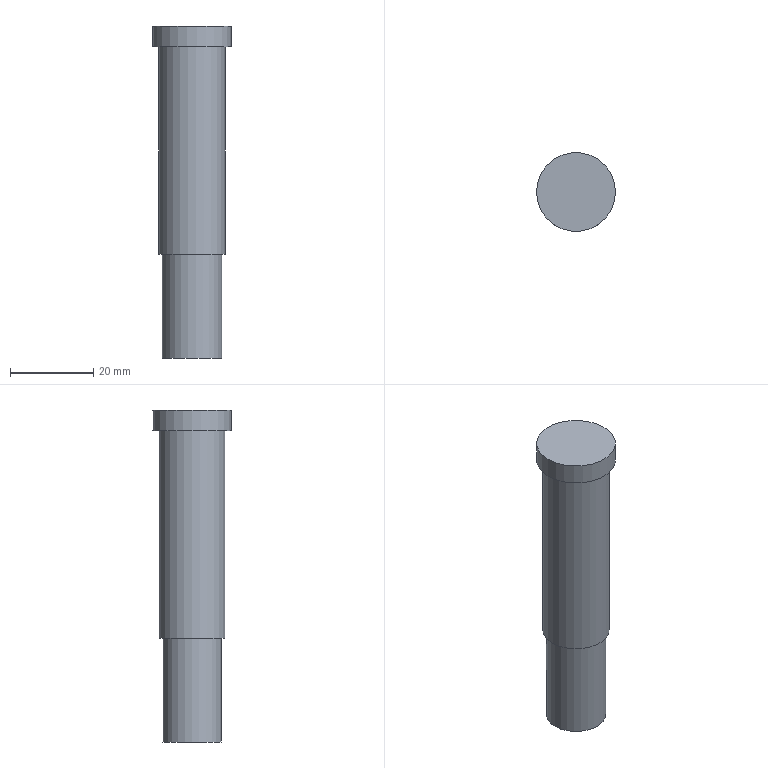Part | NX | features solid 2 | 1 solid | 7 faces | box 19 x 19 x 80 mm | volume 15486 mm3 | plane 4 | cylinder 3 | commonest cylinder face diameters 14.3 x1 16 x1 19 x1
STEP:
#1=CARTESIAN_POINT('',(-678.983,14.595,33.));
#2=VERTEX_POINT('',#1);
#3=CARTESIAN_POINT('',(-670.983,14.595,33.));
#4=DIRECTION('',(0.,0.,-1.));
#5=DIRECTION('',(-1.,0.,0.));
#6=AXIS2_PLACEMENT_3D('',#3,#4,#5);
#7=CIRCLE('',#6,8.);
#8=EDGE_CURVE('',#2,#2,#7,.T.);
#9=ORIENTED_EDGE('',*,*,#8,.F.);
#10=EDGE_LOOP('',(#9));
#11=FACE_BOUND('',#10,.T.);
#12=CARTESIAN_POINT('',(-678.983,14.595,83.));
#13=VERTEX_POINT('',#12);
#14=CARTESIAN_POINT('',(-670.983,14.595,83.));
#15=DIRECTION('',(0.,0.,-1.));
#16=DIRECTION('',(-1.,0.,0.));
#17=AXIS2_PLACEMENT_3D('',#14,#15,#16);
#18=CIRCLE('',#17,8.);
#19=EDGE_CURVE('',#13,#13,#18,.T.);
#20=ORIENTED_EDGE('',*,*,#19,.T.);
#21=EDGE_LOOP('',(#20));
#22=FACE_BOUND('',#21,.T.);
#23=CARTESIAN_POINT('',(-670.983,14.595,88.));
#24=DIRECTION('',(0.,0.,-1.));
#25=DIRECTION('',(1.,0.,0.));
#26=AXIS2_PLACEMENT_3D('',#23,#24,#25);
#27=CYLINDRICAL_SURFACE('',#26,8.);
#28=ADVANCED_FACE('',(#11,#22),#27,.T.);
#29=CARTESIAN_POINT('',(-663.833,14.595,33.));
#30=VERTEX_POINT('',#29);
#31=CARTESIAN_POINT('',(-670.983,14.595,33.));
#32=DIRECTION('',(0.,0.,1.));
#33=DIRECTION('',(1.,0.,0.));
#34=AXIS2_PLACEMENT_3D('',#31,#32,#33);
#35=CIRCLE('',#34,7.15);
#36=EDGE_CURVE('',#30,#30,#35,.T.);
#37=ORIENTED_EDGE('',*,*,#36,.T.);
#38=EDGE_LOOP('',(#37));
#39=FACE_BOUND('',#38,.T.);
#40=ORIENTED_EDGE('',*,*,#8,.T.);
#41=EDGE_LOOP('',(#40));
#42=FACE_BOUND('',#41,.T.);
#43=CARTESIAN_POINT('',(-670.983,14.595,33.));
#44=DIRECTION('',(0.,0.,1.));
#45=DIRECTION('',(-1.,0.,0.));
#46=AXIS2_PLACEMENT_3D('',#43,#44,#45);
#47=PLANE('',#46);
#48=ADVANCED_FACE('',(#39,#42),#47,.F.);
#49=CARTESIAN_POINT('',(-680.483,14.595,83.));
#50=VERTEX_POINT('',#49);
#51=CARTESIAN_POINT('',(-670.983,14.595,83.));
#52=DIRECTION('',(0.,0.,-1.));
#53=DIRECTION('',(-1.,0.,0.));
#54=AXIS2_PLACEMENT_3D('',#51,#52,#53);
#55=CIRCLE('',#54,9.5);
#56=EDGE_CURVE('',#50,#50,#55,.T.);
#57=ORIENTED_EDGE('',*,*,#56,.T.);
#58=EDGE_LOOP('',(#57));
#59=FACE_BOUND('',#58,.T.);
#60=ORIENTED_EDGE('',*,*,#19,.F.);
#61=EDGE_LOOP('',(#60));
#62=FACE_BOUND('',#61,.T.);
#63=CARTESIAN_POINT('',(-670.983,14.595,83.));
#64=DIRECTION('',(0.,0.,1.));
#65=DIRECTION('',(-1.,0.,0.));
#66=AXIS2_PLACEMENT_3D('',#63,#64,#65);
#67=PLANE('',#66);
#68=ADVANCED_FACE('',(#59,#62),#67,.F.);
#69=ORIENTED_EDGE('',*,*,#56,.F.);
#70=EDGE_LOOP('',(#69));
#71=FACE_BOUND('',#70,.T.);
#72=CARTESIAN_POINT('',(-680.483,14.595,88.));
#73=VERTEX_POINT('',#72);
#74=CARTESIAN_POINT('',(-670.983,14.595,88.));
#75=DIRECTION('',(0.,0.,-1.));
#76=DIRECTION('',(-1.,0.,0.));
#77=AXIS2_PLACEMENT_3D('',#74,#75,#76);
#78=CIRCLE('',#77,9.5);
#79=EDGE_CURVE('',#73,#73,#78,.T.);
#80=ORIENTED_EDGE('',*,*,#79,.T.);
#81=EDGE_LOOP('',(#80));
#82=FACE_BOUND('',#81,.T.);
#83=CARTESIAN_POINT('',(-670.983,14.595,83.));
#84=DIRECTION('',(0.,0.,1.));
#85=DIRECTION('',(-1.,0.,0.));
#86=AXIS2_PLACEMENT_3D('',#83,#84,#85);
#87=CYLINDRICAL_SURFACE('',#86,9.5);
#88=ADVANCED_FACE('',(#71,#82),#87,.T.);
#89=ORIENTED_EDGE('',*,*,#79,.F.);
#90=EDGE_LOOP('',(#89));
#91=FACE_BOUND('',#90,.T.);
#92=CARTESIAN_POINT('',(-670.983,14.595,88.));
#93=DIRECTION('',(0.,0.,1.));
#94=DIRECTION('',(-1.,0.,0.));
#95=AXIS2_PLACEMENT_3D('',#92,#93,#94);
#96=PLANE('',#95);
#97=ADVANCED_FACE('',(#91),#96,.T.);
#98=CARTESIAN_POINT('',(-663.833,14.595,8.));
#99=VERTEX_POINT('',#98);
#100=CARTESIAN_POINT('',(-670.983,14.595,8.));
#101=DIRECTION('',(0.,0.,1.));
#102=DIRECTION('',(1.,0.,0.));
#103=AXIS2_PLACEMENT_3D('',#100,#101,#102);
#104=CIRCLE('',#103,7.15);
#105=EDGE_CURVE('',#99,#99,#104,.T.);
#106=ORIENTED_EDGE('',*,*,#105,.T.);
#107=EDGE_LOOP('',(#106));
#108=FACE_BOUND('',#107,.T.);
#109=ORIENTED_EDGE('',*,*,#36,.F.);
#110=EDGE_LOOP('',(#109));
#111=FACE_BOUND('',#110,.T.);
#112=CARTESIAN_POINT('',(-670.983,14.595,8.));
#113=DIRECTION('',(0.,0.,1.));
#114=DIRECTION('',(1.,0.,0.));
#115=AXIS2_PLACEMENT_3D('',#112,#113,#114);
#116=CYLINDRICAL_SURFACE('',#115,7.15);
#117=ADVANCED_FACE('',(#108,#111),#116,.T.);
#118=ORIENTED_EDGE('',*,*,#105,.F.);
#119=EDGE_LOOP('',(#118));
#120=FACE_BOUND('',#119,.T.);
#121=CARTESIAN_POINT('',(-670.983,14.595,8.));
#122=DIRECTION('',(0.,0.,1.));
#123=DIRECTION('',(-1.,0.,0.));
#124=AXIS2_PLACEMENT_3D('',#121,#122,#123);
#125=PLANE('',#124);
#126=ADVANCED_FACE('',(#120),#125,.F.);
#127=CLOSED_SHELL('',(#28,#48,#68,#88,#97,#117,#126));
#128=MANIFOLD_SOLID_BREP('',#127);
#129=(LENGTH_UNIT()NAMED_UNIT(*)SI_UNIT(.MILLI.,.METRE.));
#130=UNCERTAINTY_MEASURE_WITH_UNIT(LENGTH_MEASURE(0.00001),#129,'','');
#131=(NAMED_UNIT(*)PLANE_ANGLE_UNIT()SI_UNIT($,.RADIAN.));
#132=(NAMED_UNIT(*)SI_UNIT($,.STERADIAN.)SOLID_ANGLE_UNIT());
#133=(GEOMETRIC_REPRESENTATION_CONTEXT(3)GLOBAL_UNCERTAINTY_ASSIGNED_CONTEXT((#130))GLOBAL_UNIT_ASSIGNED_CONTEXT((#129,#131,#132))REPRESENTATION_CONTEXT('',''));
#134=ADVANCED_BREP_SHAPE_REPRESENTATION('',(#128),#133);